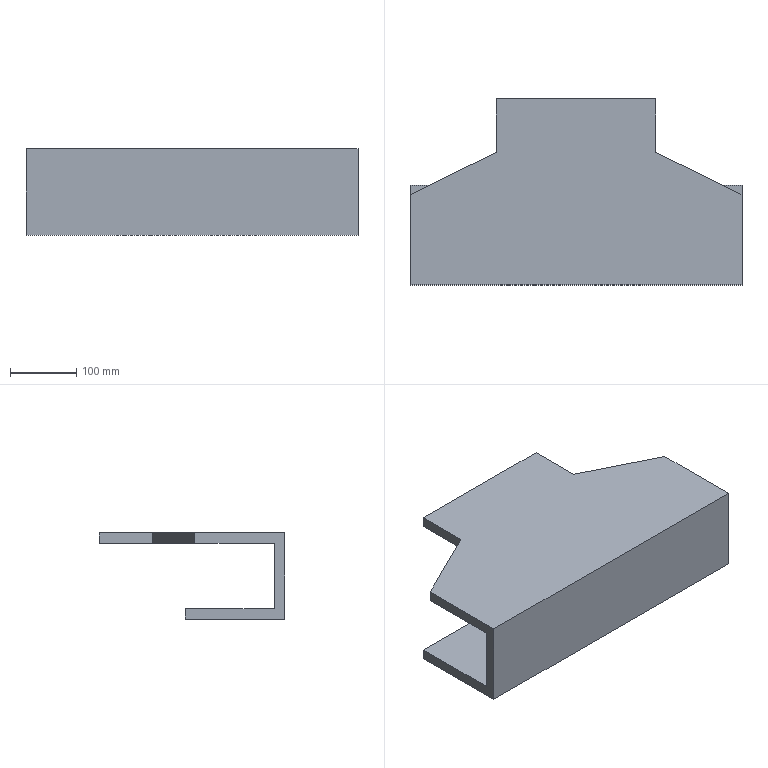Part | SolidWorks | features ICE 2, Extrusion 1 | 1 solid | 14 faces | box 500 x 280 x 130 mm | volume 3757451 mm3 | plane 14
STEP:
#1=CARTESIAN_POINT('',(120.,200.,0.));
#2=VERTEX_POINT('',#1);
#3=CARTESIAN_POINT('',(120.,280.,0.));
#4=VERTEX_POINT('',#3);
#5=CARTESIAN_POINT('',(120.,280.,0.));
#6=DIRECTION('',(0.,1.,0.));
#7=VECTOR('',#6,1000.);
#8=LINE('',#5,#7);
#9=EDGE_CURVE('',#2,#4,#8,.T.);
#10=ORIENTED_EDGE('',*,*,#9,.T.);
#11=CARTESIAN_POINT('',(120.,280.,16.));
#12=VERTEX_POINT('',#11);
#13=CARTESIAN_POINT('',(120.,280.,16.));
#14=DIRECTION('',(0.,0.,-1.));
#15=VECTOR('',#14,1000.);
#16=LINE('',#13,#15);
#17=EDGE_CURVE('',#12,#4,#16,.T.);
#18=ORIENTED_EDGE('',*,*,#17,.F.);
#19=CARTESIAN_POINT('',(120.,200.,16.));
#20=VERTEX_POINT('',#19);
#21=CARTESIAN_POINT('',(120.,280.,16.));
#22=DIRECTION('',(0.,1.,0.));
#23=VECTOR('',#22,1000.);
#24=LINE('',#21,#23);
#25=EDGE_CURVE('',#20,#12,#24,.T.);
#26=ORIENTED_EDGE('',*,*,#25,.F.);
#27=CARTESIAN_POINT('',(120.,200.,16.));
#28=DIRECTION('',(0.,0.,-1.));
#29=VECTOR('',#28,1000.);
#30=LINE('',#27,#29);
#31=EDGE_CURVE('',#20,#2,#30,.T.);
#32=ORIENTED_EDGE('',*,*,#31,.T.);
#33=EDGE_LOOP('',(#10,#18,#26,#32));
#34=FACE_OUTER_BOUND('',#33,.T.);
#35=CARTESIAN_POINT('',(120.,280.,16.));
#36=DIRECTION('',(-1.,0.,0.));
#37=DIRECTION('',(0.,0.,1.));
#38=AXIS2_PLACEMENT_3D('',#35,#36,#37);
#39=PLANE('',#38);
#40=ADVANCED_FACE('',(#34),#39,.F.);
#41=CARTESIAN_POINT('',(-120.,280.,0.));
#42=VERTEX_POINT('',#41);
#43=CARTESIAN_POINT('',(120.,280.,0.));
#44=DIRECTION('',(-1.,0.,0.));
#45=VECTOR('',#44,1000.);
#46=LINE('',#43,#45);
#47=EDGE_CURVE('',#4,#42,#46,.T.);
#48=ORIENTED_EDGE('',*,*,#47,.T.);
#49=CARTESIAN_POINT('',(-120.,280.,16.));
#50=VERTEX_POINT('',#49);
#51=CARTESIAN_POINT('',(-120.,280.,16.));
#52=DIRECTION('',(0.,0.,-1.));
#53=VECTOR('',#52,1000.);
#54=LINE('',#51,#53);
#55=EDGE_CURVE('',#50,#42,#54,.T.);
#56=ORIENTED_EDGE('',*,*,#55,.F.);
#57=CARTESIAN_POINT('',(120.,280.,16.));
#58=DIRECTION('',(-1.,0.,0.));
#59=VECTOR('',#58,1000.);
#60=LINE('',#57,#59);
#61=EDGE_CURVE('',#12,#50,#60,.T.);
#62=ORIENTED_EDGE('',*,*,#61,.F.);
#63=ORIENTED_EDGE('',*,*,#17,.T.);
#64=EDGE_LOOP('',(#48,#56,#62,#63));
#65=FACE_OUTER_BOUND('',#64,.T.);
#66=CARTESIAN_POINT('',(120.,280.,16.));
#67=DIRECTION('',(0.,-1.,0.));
#68=DIRECTION('',(0.,0.,-1.));
#69=AXIS2_PLACEMENT_3D('',#66,#67,#68);
#70=PLANE('',#69);
#71=ADVANCED_FACE('',(#65),#70,.F.);
#72=CARTESIAN_POINT('',(-120.,200.,0.));
#73=VERTEX_POINT('',#72);
#74=CARTESIAN_POINT('',(-120.,280.,0.));
#75=DIRECTION('',(0.,-1.,0.));
#76=VECTOR('',#75,1000.);
#77=LINE('',#74,#76);
#78=EDGE_CURVE('',#42,#73,#77,.T.);
#79=ORIENTED_EDGE('',*,*,#78,.T.);
#80=CARTESIAN_POINT('',(-120.,200.,16.));
#81=VERTEX_POINT('',#80);
#82=CARTESIAN_POINT('',(-120.,200.,16.));
#83=DIRECTION('',(0.,0.,-1.));
#84=VECTOR('',#83,1000.);
#85=LINE('',#82,#84);
#86=EDGE_CURVE('',#81,#73,#85,.T.);
#87=ORIENTED_EDGE('',*,*,#86,.F.);
#88=CARTESIAN_POINT('',(-120.,280.,16.));
#89=DIRECTION('',(0.,-1.,0.));
#90=VECTOR('',#89,1000.);
#91=LINE('',#88,#90);
#92=EDGE_CURVE('',#50,#81,#91,.T.);
#93=ORIENTED_EDGE('',*,*,#92,.F.);
#94=ORIENTED_EDGE('',*,*,#55,.T.);
#95=EDGE_LOOP('',(#79,#87,#93,#94));
#96=FACE_OUTER_BOUND('',#95,.T.);
#97=CARTESIAN_POINT('',(-120.,280.,16.));
#98=DIRECTION('',(1.,0.,0.));
#99=DIRECTION('',(0.,0.,-1.));
#100=AXIS2_PLACEMENT_3D('',#97,#98,#99);
#101=PLANE('',#100);
#102=ADVANCED_FACE('',(#96),#101,.F.);
#103=CARTESIAN_POINT('',(-250.,135.698,0.));
#104=VERTEX_POINT('',#103);
#105=CARTESIAN_POINT('',(-120.,200.,0.));
#106=DIRECTION('',(-0.8963,-0.4434,0.));
#107=VECTOR('',#106,1000.);
#108=LINE('',#105,#107);
#109=EDGE_CURVE('',#73,#104,#108,.T.);
#110=ORIENTED_EDGE('',*,*,#109,.T.);
#111=CARTESIAN_POINT('',(-250.,135.698,16.));
#112=VERTEX_POINT('',#111);
#113=CARTESIAN_POINT('',(-250.,135.698,16.));
#114=DIRECTION('',(0.,0.,-1.));
#115=VECTOR('',#114,1000.);
#116=LINE('',#113,#115);
#117=EDGE_CURVE('',#112,#104,#116,.T.);
#118=ORIENTED_EDGE('',*,*,#117,.F.);
#119=CARTESIAN_POINT('',(-120.,200.,16.));
#120=DIRECTION('',(-0.8963,-0.4434,0.));
#121=VECTOR('',#120,1000.);
#122=LINE('',#119,#121);
#123=EDGE_CURVE('',#81,#112,#122,.T.);
#124=ORIENTED_EDGE('',*,*,#123,.F.);
#125=ORIENTED_EDGE('',*,*,#86,.T.);
#126=EDGE_LOOP('',(#110,#118,#124,#125));
#127=FACE_OUTER_BOUND('',#126,.T.);
#128=CARTESIAN_POINT('',(-120.,200.,16.));
#129=DIRECTION('',(0.4434,-0.8963,0.));
#130=DIRECTION('',(0.8963,0.4434,0.));
#131=AXIS2_PLACEMENT_3D('',#128,#129,#130);
#132=PLANE('',#131);
#133=ADVANCED_FACE('',(#127),#132,.F.);
#134=CARTESIAN_POINT('',(-250.,16.,-98.));
#135=VERTEX_POINT('',#134);
#136=CARTESIAN_POINT('',(-250.,16.,0.));
#137=VERTEX_POINT('',#136);
#138=CARTESIAN_POINT('',(-250.,16.,-114.));
#139=DIRECTION('',(0.,0.,1.));
#140=VECTOR('',#139,1000.);
#141=LINE('',#138,#140);
#142=EDGE_CURVE('',#135,#137,#141,.T.);
#143=ORIENTED_EDGE('',*,*,#142,.F.);
#144=CARTESIAN_POINT('',(-250.,150.,-98.));
#145=VERTEX_POINT('',#144);
#146=CARTESIAN_POINT('',(-250.,150.,-98.));
#147=DIRECTION('',(0.,-1.,0.));
#148=VECTOR('',#147,1000.);
#149=LINE('',#146,#148);
#150=EDGE_CURVE('',#145,#135,#149,.T.);
#151=ORIENTED_EDGE('',*,*,#150,.F.);
#152=CARTESIAN_POINT('',(-250.,150.,-114.));
#153=VERTEX_POINT('',#152);
#154=CARTESIAN_POINT('',(-250.,150.,-98.));
#155=DIRECTION('',(0.,0.,-1.));
#156=VECTOR('',#155,1000.);
#157=LINE('',#154,#156);
#158=EDGE_CURVE('',#145,#153,#157,.T.);
#159=ORIENTED_EDGE('',*,*,#158,.T.);
#160=CARTESIAN_POINT('',(-250.,0.,-114.));
#161=VERTEX_POINT('',#160);
#162=CARTESIAN_POINT('',(-250.,16.,-114.));
#163=DIRECTION('',(0.,-1.,0.));
#164=VECTOR('',#163,1000.);
#165=LINE('',#162,#164);
#166=EDGE_CURVE('',#153,#161,#165,.T.);
#167=ORIENTED_EDGE('',*,*,#166,.T.);
#168=CARTESIAN_POINT('',(-250.,0.,16.));
#169=VERTEX_POINT('',#168);
#170=CARTESIAN_POINT('',(-250.,0.,16.));
#171=DIRECTION('',(0.,0.,-1.));
#172=VECTOR('',#171,1000.);
#173=LINE('',#170,#172);
#174=EDGE_CURVE('',#169,#161,#173,.T.);
#175=ORIENTED_EDGE('',*,*,#174,.F.);
#176=CARTESIAN_POINT('',(-250.,135.698,16.));
#177=DIRECTION('',(0.,-1.,0.));
#178=VECTOR('',#177,1000.);
#179=LINE('',#176,#178);
#180=EDGE_CURVE('',#112,#169,#179,.T.);
#181=ORIENTED_EDGE('',*,*,#180,.F.);
#182=ORIENTED_EDGE('',*,*,#117,.T.);
#183=CARTESIAN_POINT('',(-250.,135.698,0.));
#184=DIRECTION('',(0.,-1.,0.));
#185=VECTOR('',#184,1000.);
#186=LINE('',#183,#185);
#187=EDGE_CURVE('',#104,#137,#186,.T.);
#188=ORIENTED_EDGE('',*,*,#187,.T.);
#189=EDGE_LOOP('',(#143,#151,#159,#167,#175,#181,#182,#188));
#190=FACE_OUTER_BOUND('',#189,.T.);
#191=CARTESIAN_POINT('',(-250.,135.698,16.));
#192=DIRECTION('',(1.,0.,0.));
#193=DIRECTION('',(0.,0.,-1.));
#194=AXIS2_PLACEMENT_3D('',#191,#192,#193);
#195=PLANE('',#194);
#196=ADVANCED_FACE('',(#190),#195,.F.);
#197=ORIENTED_EDGE('',*,*,#174,.T.);
#198=CARTESIAN_POINT('',(250.,0.,-114.));
#199=VERTEX_POINT('',#198);
#200=CARTESIAN_POINT('',(-250.,0.,-114.));
#201=DIRECTION('',(1.,0.,0.));
#202=VECTOR('',#201,1000.);
#203=LINE('',#200,#202);
#204=EDGE_CURVE('',#161,#199,#203,.T.);
#205=ORIENTED_EDGE('',*,*,#204,.T.);
#206=CARTESIAN_POINT('',(250.,0.,16.));
#207=VERTEX_POINT('',#206);
#208=CARTESIAN_POINT('',(250.,0.,16.));
#209=DIRECTION('',(0.,0.,-1.));
#210=VECTOR('',#209,1000.);
#211=LINE('',#208,#210);
#212=EDGE_CURVE('',#207,#199,#211,.T.);
#213=ORIENTED_EDGE('',*,*,#212,.F.);
#214=CARTESIAN_POINT('',(-250.,0.,16.));
#215=DIRECTION('',(1.,0.,0.));
#216=VECTOR('',#215,1000.);
#217=LINE('',#214,#216);
#218=EDGE_CURVE('',#169,#207,#217,.T.);
#219=ORIENTED_EDGE('',*,*,#218,.F.);
#220=EDGE_LOOP('',(#197,#205,#213,#219));
#221=FACE_OUTER_BOUND('',#220,.T.);
#222=CARTESIAN_POINT('',(-250.,0.,16.));
#223=DIRECTION('',(0.,1.,0.));
#224=DIRECTION('',(0.,0.,1.));
#225=AXIS2_PLACEMENT_3D('',#222,#223,#224);
#226=PLANE('',#225);
#227=ADVANCED_FACE('',(#221),#226,.F.);
#228=ORIENTED_EDGE('',*,*,#212,.T.);
#229=CARTESIAN_POINT('',(250.,150.,-114.));
#230=VERTEX_POINT('',#229);
#231=CARTESIAN_POINT('',(250.,16.,-114.));
#232=DIRECTION('',(0.,1.,0.));
#233=VECTOR('',#232,1000.);
#234=LINE('',#231,#233);
#235=EDGE_CURVE('',#199,#230,#234,.T.);
#236=ORIENTED_EDGE('',*,*,#235,.T.);
#237=CARTESIAN_POINT('',(250.,150.,-98.));
#238=VERTEX_POINT('',#237);
#239=CARTESIAN_POINT('',(250.,150.,-98.));
#240=DIRECTION('',(0.,0.,1.));
#241=VECTOR('',#240,1000.);
#242=LINE('',#239,#241);
#243=EDGE_CURVE('',#230,#238,#242,.T.);
#244=ORIENTED_EDGE('',*,*,#243,.T.);
#245=CARTESIAN_POINT('',(250.,16.,-98.));
#246=VERTEX_POINT('',#245);
#247=CARTESIAN_POINT('',(250.,150.,-98.));
#248=DIRECTION('',(0.,-1.,0.));
#249=VECTOR('',#248,1000.);
#250=LINE('',#247,#249);
#251=EDGE_CURVE('',#238,#246,#250,.T.);
#252=ORIENTED_EDGE('',*,*,#251,.T.);
#253=CARTESIAN_POINT('',(250.,16.,0.));
#254=VERTEX_POINT('',#253);
#255=CARTESIAN_POINT('',(250.,16.,-114.));
#256=DIRECTION('',(0.,0.,1.));
#257=VECTOR('',#256,1000.);
#258=LINE('',#255,#257);
#259=EDGE_CURVE('',#246,#254,#258,.T.);
#260=ORIENTED_EDGE('',*,*,#259,.T.);
#261=CARTESIAN_POINT('',(250.,135.698,0.));
#262=VERTEX_POINT('',#261);
#263=CARTESIAN_POINT('',(250.,135.698,0.));
#264=DIRECTION('',(0.,1.,0.));
#265=VECTOR('',#264,1000.);
#266=LINE('',#263,#265);
#267=EDGE_CURVE('',#254,#262,#266,.T.);
#268=ORIENTED_EDGE('',*,*,#267,.T.);
#269=CARTESIAN_POINT('',(250.,135.698,16.));
#270=VERTEX_POINT('',#269);
#271=CARTESIAN_POINT('',(250.,135.698,16.));
#272=DIRECTION('',(0.,0.,-1.));
#273=VECTOR('',#272,1000.);
#274=LINE('',#271,#273);
#275=EDGE_CURVE('',#270,#262,#274,.T.);
#276=ORIENTED_EDGE('',*,*,#275,.F.);
#277=CARTESIAN_POINT('',(250.,135.698,16.));
#278=DIRECTION('',(0.,1.,0.));
#279=VECTOR('',#278,1000.);
#280=LINE('',#277,#279);
#281=EDGE_CURVE('',#207,#270,#280,.T.);
#282=ORIENTED_EDGE('',*,*,#281,.F.);
#283=EDGE_LOOP('',(#228,#236,#244,#252,#260,#268,#276,#282));
#284=FACE_OUTER_BOUND('',#283,.T.);
#285=CARTESIAN_POINT('',(250.,135.698,16.));
#286=DIRECTION('',(-1.,0.,0.));
#287=DIRECTION('',(0.,0.,1.));
#288=AXIS2_PLACEMENT_3D('',#285,#286,#287);
#289=PLANE('',#288);
#290=ADVANCED_FACE('',(#284),#289,.F.);
#291=CARTESIAN_POINT('',(120.,200.,0.));
#292=DIRECTION('',(-0.8963,0.4434,0.));
#293=VECTOR('',#292,1000.);
#294=LINE('',#291,#293);
#295=EDGE_CURVE('',#262,#2,#294,.T.);
#296=ORIENTED_EDGE('',*,*,#295,.T.);
#297=ORIENTED_EDGE('',*,*,#31,.F.);
#298=CARTESIAN_POINT('',(120.,200.,16.));
#299=DIRECTION('',(-0.8963,0.4434,0.));
#300=VECTOR('',#299,1000.);
#301=LINE('',#298,#300);
#302=EDGE_CURVE('',#270,#20,#301,.T.);
#303=ORIENTED_EDGE('',*,*,#302,.F.);
#304=ORIENTED_EDGE('',*,*,#275,.T.);
#305=EDGE_LOOP('',(#296,#297,#303,#304));
#306=FACE_OUTER_BOUND('',#305,.T.);
#307=CARTESIAN_POINT('',(120.,200.,16.));
#308=DIRECTION('',(-0.4434,-0.8963,0.));
#309=DIRECTION('',(0.8963,-0.4434,0.));
#310=AXIS2_PLACEMENT_3D('',#307,#308,#309);
#311=PLANE('',#310);
#312=ADVANCED_FACE('',(#306),#311,.F.);
#313=ORIENTED_EDGE('',*,*,#180,.T.);
#314=ORIENTED_EDGE('',*,*,#218,.T.);
#315=ORIENTED_EDGE('',*,*,#281,.T.);
#316=ORIENTED_EDGE('',*,*,#302,.T.);
#317=ORIENTED_EDGE('',*,*,#25,.T.);
#318=ORIENTED_EDGE('',*,*,#61,.T.);
#319=ORIENTED_EDGE('',*,*,#92,.T.);
#320=ORIENTED_EDGE('',*,*,#123,.T.);
#321=EDGE_LOOP('',(#313,#314,#315,#316,#317,#318,#319,#320));
#322=FACE_OUTER_BOUND('',#321,.T.);
#323=CARTESIAN_POINT('',(0.,0.,16.));
#324=DIRECTION('',(0.,0.,1.));
#325=DIRECTION('',(1.,0.,0.));
#326=AXIS2_PLACEMENT_3D('',#323,#324,#325);
#327=PLANE('',#326);
#328=ADVANCED_FACE('',(#322),#327,.T.);
#329=ORIENTED_EDGE('',*,*,#267,.F.);
#330=CARTESIAN_POINT('',(0.,16.,0.));
#331=DIRECTION('',(-1.,0.,0.));
#332=VECTOR('',#331,1000.);
#333=LINE('',#330,#332);
#334=EDGE_CURVE('',#254,#137,#333,.T.);
#335=ORIENTED_EDGE('',*,*,#334,.T.);
#336=ORIENTED_EDGE('',*,*,#187,.F.);
#337=ORIENTED_EDGE('',*,*,#109,.F.);
#338=ORIENTED_EDGE('',*,*,#78,.F.);
#339=ORIENTED_EDGE('',*,*,#47,.F.);
#340=ORIENTED_EDGE('',*,*,#9,.F.);
#341=ORIENTED_EDGE('',*,*,#295,.F.);
#342=EDGE_LOOP('',(#329,#335,#336,#337,#338,#339,#340,#341));
#343=FACE_OUTER_BOUND('',#342,.T.);
#344=CARTESIAN_POINT('',(0.,0.,0.));
#345=DIRECTION('',(0.,0.,1.));
#346=DIRECTION('',(1.,0.,0.));
#347=AXIS2_PLACEMENT_3D('',#344,#345,#346);
#348=PLANE('',#347);
#349=ADVANCED_FACE('',(#343),#348,.F.);
#350=CARTESIAN_POINT('',(-250.,16.,-98.));
#351=DIRECTION('',(1.,0.,0.));
#352=VECTOR('',#351,1000.);
#353=LINE('',#350,#352);
#354=EDGE_CURVE('',#135,#246,#353,.T.);
#355=ORIENTED_EDGE('',*,*,#354,.F.);
#356=ORIENTED_EDGE('',*,*,#142,.T.);
#357=ORIENTED_EDGE('',*,*,#334,.F.);
#358=ORIENTED_EDGE('',*,*,#259,.F.);
#359=EDGE_LOOP('',(#355,#356,#357,#358));
#360=FACE_OUTER_BOUND('',#359,.T.);
#361=CARTESIAN_POINT('',(-250.,16.,-114.));
#362=DIRECTION('',(0.,1.,0.));
#363=DIRECTION('',(0.,0.,1.));
#364=AXIS2_PLACEMENT_3D('',#361,#362,#363);
#365=PLANE('',#364);
#366=ADVANCED_FACE('',(#360),#365,.T.);
#367=ORIENTED_EDGE('',*,*,#235,.F.);
#368=ORIENTED_EDGE('',*,*,#204,.F.);
#369=ORIENTED_EDGE('',*,*,#166,.F.);
#370=CARTESIAN_POINT('',(-250.,150.,-114.));
#371=DIRECTION('',(1.,0.,0.));
#372=VECTOR('',#371,1000.);
#373=LINE('',#370,#372);
#374=EDGE_CURVE('',#153,#230,#373,.T.);
#375=ORIENTED_EDGE('',*,*,#374,.T.);
#376=EDGE_LOOP('',(#367,#368,#369,#375));
#377=FACE_OUTER_BOUND('',#376,.T.);
#378=CARTESIAN_POINT('',(0.,0.,-114.));
#379=DIRECTION('',(0.,0.,1.));
#380=DIRECTION('',(1.,0.,0.));
#381=AXIS2_PLACEMENT_3D('',#378,#379,#380);
#382=PLANE('',#381);
#383=ADVANCED_FACE('',(#377),#382,.F.);
#384=ORIENTED_EDGE('',*,*,#150,.T.);
#385=ORIENTED_EDGE('',*,*,#354,.T.);
#386=ORIENTED_EDGE('',*,*,#251,.F.);
#387=CARTESIAN_POINT('',(-250.,150.,-98.));
#388=DIRECTION('',(-1.,0.,0.));
#389=VECTOR('',#388,1000.);
#390=LINE('',#387,#389);
#391=EDGE_CURVE('',#238,#145,#390,.T.);
#392=ORIENTED_EDGE('',*,*,#391,.T.);
#393=EDGE_LOOP('',(#384,#385,#386,#392));
#394=FACE_OUTER_BOUND('',#393,.T.);
#395=CARTESIAN_POINT('',(-250.,150.,-98.));
#396=DIRECTION('',(0.,0.,1.));
#397=DIRECTION('',(1.,0.,0.));
#398=AXIS2_PLACEMENT_3D('',#395,#396,#397);
#399=PLANE('',#398);
#400=ADVANCED_FACE('',(#394),#399,.T.);
#401=ORIENTED_EDGE('',*,*,#243,.F.);
#402=ORIENTED_EDGE('',*,*,#374,.F.);
#403=ORIENTED_EDGE('',*,*,#158,.F.);
#404=ORIENTED_EDGE('',*,*,#391,.F.);
#405=EDGE_LOOP('',(#401,#402,#403,#404));
#406=FACE_OUTER_BOUND('',#405,.T.);
#407=CARTESIAN_POINT('',(0.,150.,0.));
#408=DIRECTION('',(0.,-1.,0.));
#409=DIRECTION('',(0.,0.,-1.));
#410=AXIS2_PLACEMENT_3D('',#407,#408,#409);
#411=PLANE('',#410);
#412=ADVANCED_FACE('',(#406),#411,.F.);
#413=CLOSED_SHELL('',(#40,#71,#102,#133,#196,#227,#290,#312,#328,#349,#366,#383,#400,#412));
#414=MANIFOLD_SOLID_BREP('',#413);
#415=CARTESIAN_POINT('',(0.,0.,0.));
#416=DIRECTION('',(0.,0.,1.));
#417=DIRECTION('',(1.,0.,0.));
#418=AXIS2_PLACEMENT_3D('',#415,#416,#417);
#419=(LENGTH_UNIT()NAMED_UNIT(*)SI_UNIT(.MILLI.,.METRE.));
#420=UNCERTAINTY_MEASURE_WITH_UNIT(LENGTH_MEASURE(0.00001),#419,'','');
#421=(NAMED_UNIT(*)PLANE_ANGLE_UNIT()SI_UNIT($,.RADIAN.));
#422=(NAMED_UNIT(*)SI_UNIT($,.STERADIAN.)SOLID_ANGLE_UNIT());
#423=(GEOMETRIC_REPRESENTATION_CONTEXT(3)GLOBAL_UNCERTAINTY_ASSIGNED_CONTEXT((#420))GLOBAL_UNIT_ASSIGNED_CONTEXT((#419,#421,#422))REPRESENTATION_CONTEXT('',''));
#424=ADVANCED_BREP_SHAPE_REPRESENTATION('',(#414,#418),#423);